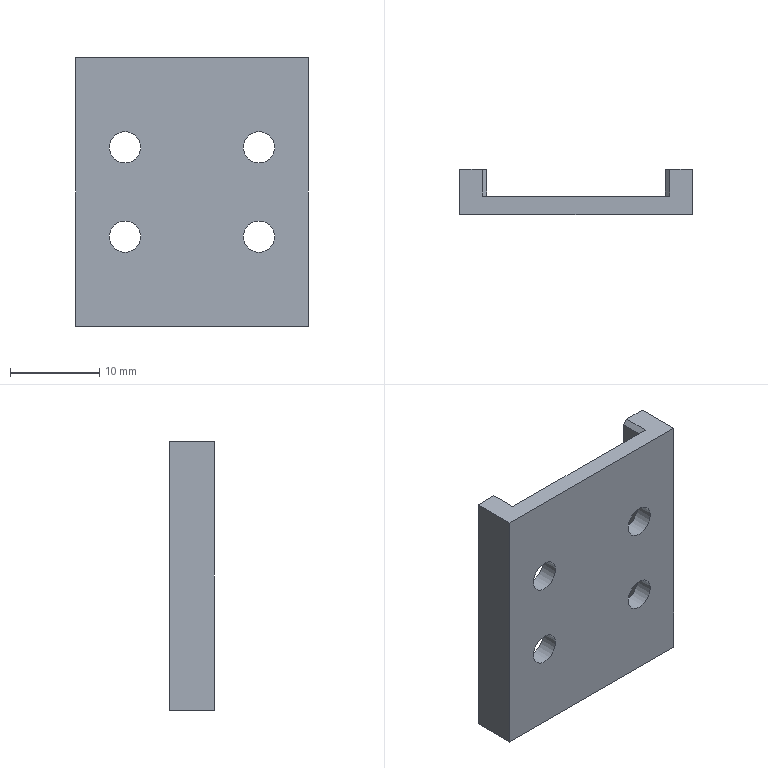Part | NX | 1 solid | 18 faces | box 26 x 5 x 30 mm | volume 2030 mm3 | plane 14 | cylinder 4 | commonest cylinder face diameters 3.5 x4
STEP:
#1=CARTESIAN_POINT('',(-13.,2.5,-15.));
#2=VERTEX_POINT('',#1);
#3=CARTESIAN_POINT('',(-13.,-2.5,-15.));
#4=VERTEX_POINT('',#3);
#5=CARTESIAN_POINT('',(-13.,2.5,-15.));
#6=DIRECTION('',(0.,-1.,0.));
#7=VECTOR('',#6,1000.);
#8=LINE('',#5,#7);
#9=EDGE_CURVE('',#2,#4,#8,.T.);
#10=ORIENTED_EDGE('',*,*,#9,.T.);
#11=CARTESIAN_POINT('',(-13.,-2.5,15.));
#12=VERTEX_POINT('',#11);
#13=CARTESIAN_POINT('',(-13.,-2.5,15.));
#14=DIRECTION('',(0.,0.,-1.));
#15=VECTOR('',#14,1000.);
#16=LINE('',#13,#15);
#17=EDGE_CURVE('',#12,#4,#16,.T.);
#18=ORIENTED_EDGE('',*,*,#17,.F.);
#19=CARTESIAN_POINT('',(-13.,2.5,15.));
#20=VERTEX_POINT('',#19);
#21=CARTESIAN_POINT('',(-13.,2.5,15.));
#22=DIRECTION('',(0.,-1.,0.));
#23=VECTOR('',#22,1000.);
#24=LINE('',#21,#23);
#25=EDGE_CURVE('',#20,#12,#24,.T.);
#26=ORIENTED_EDGE('',*,*,#25,.F.);
#27=CARTESIAN_POINT('',(-13.,2.5,15.));
#28=DIRECTION('',(0.,0.,-1.));
#29=VECTOR('',#28,1000.);
#30=LINE('',#27,#29);
#31=EDGE_CURVE('',#20,#2,#30,.T.);
#32=ORIENTED_EDGE('',*,*,#31,.T.);
#33=EDGE_LOOP('',(#10,#18,#26,#32));
#34=FACE_BOUND('',#33,.T.);
#35=CARTESIAN_POINT('',(-13.,2.5,15.));
#36=DIRECTION('',(1.,0.,0.));
#37=DIRECTION('',(0.,0.,-1.));
#38=AXIS2_PLACEMENT_3D('',#35,#36,#37);
#39=PLANE('',#38);
#40=ADVANCED_FACE('',(#34),#39,.F.);
#41=CARTESIAN_POINT('',(7.5,-2.5,-3.25));
#42=VERTEX_POINT('',#41);
#43=CARTESIAN_POINT('',(7.5,-2.5,-5.));
#44=DIRECTION('',(0.,1.,0.));
#45=DIRECTION('',(0.,0.,1.));
#46=AXIS2_PLACEMENT_3D('',#43,#44,#45);
#47=CIRCLE('',#46,1.75);
#48=EDGE_CURVE('',#42,#42,#47,.F.);
#49=ORIENTED_EDGE('',*,*,#48,.F.);
#50=EDGE_LOOP('',(#49));
#51=FACE_BOUND('',#50,.T.);
#52=CARTESIAN_POINT('',(-7.5,-2.5,6.75));
#53=VERTEX_POINT('',#52);
#54=CARTESIAN_POINT('',(-7.5,-2.5,5.));
#55=DIRECTION('',(0.,1.,0.));
#56=DIRECTION('',(0.,0.,1.));
#57=AXIS2_PLACEMENT_3D('',#54,#55,#56);
#58=CIRCLE('',#57,1.75);
#59=EDGE_CURVE('',#53,#53,#58,.F.);
#60=ORIENTED_EDGE('',*,*,#59,.F.);
#61=EDGE_LOOP('',(#60));
#62=FACE_BOUND('',#61,.T.);
#63=CARTESIAN_POINT('',(-7.5,-2.5,-3.25));
#64=VERTEX_POINT('',#63);
#65=CARTESIAN_POINT('',(-7.5,-2.5,-5.));
#66=DIRECTION('',(0.,1.,0.));
#67=DIRECTION('',(0.,0.,1.));
#68=AXIS2_PLACEMENT_3D('',#65,#66,#67);
#69=CIRCLE('',#68,1.75);
#70=EDGE_CURVE('',#64,#64,#69,.F.);
#71=ORIENTED_EDGE('',*,*,#70,.F.);
#72=EDGE_LOOP('',(#71));
#73=FACE_BOUND('',#72,.T.);
#74=CARTESIAN_POINT('',(7.5,-2.5,6.75));
#75=VERTEX_POINT('',#74);
#76=CARTESIAN_POINT('',(7.5,-2.5,5.));
#77=DIRECTION('',(0.,1.,0.));
#78=DIRECTION('',(0.,0.,1.));
#79=AXIS2_PLACEMENT_3D('',#76,#77,#78);
#80=CIRCLE('',#79,1.75);
#81=EDGE_CURVE('',#75,#75,#80,.F.);
#82=ORIENTED_EDGE('',*,*,#81,.F.);
#83=EDGE_LOOP('',(#82));
#84=FACE_BOUND('',#83,.T.);
#85=CARTESIAN_POINT('',(13.,-2.5,-15.));
#86=VERTEX_POINT('',#85);
#87=CARTESIAN_POINT('',(-13.,-2.5,-15.));
#88=DIRECTION('',(1.,0.,0.));
#89=VECTOR('',#88,1000.);
#90=LINE('',#87,#89);
#91=EDGE_CURVE('',#4,#86,#90,.T.);
#92=ORIENTED_EDGE('',*,*,#91,.T.);
#93=CARTESIAN_POINT('',(13.,-2.5,15.));
#94=VERTEX_POINT('',#93);
#95=CARTESIAN_POINT('',(13.,-2.5,15.));
#96=DIRECTION('',(0.,0.,-1.));
#97=VECTOR('',#96,1000.);
#98=LINE('',#95,#97);
#99=EDGE_CURVE('',#94,#86,#98,.T.);
#100=ORIENTED_EDGE('',*,*,#99,.F.);
#101=CARTESIAN_POINT('',(-13.,-2.5,15.));
#102=DIRECTION('',(1.,0.,0.));
#103=VECTOR('',#102,1000.);
#104=LINE('',#101,#103);
#105=EDGE_CURVE('',#12,#94,#104,.T.);
#106=ORIENTED_EDGE('',*,*,#105,.F.);
#107=ORIENTED_EDGE('',*,*,#17,.T.);
#108=EDGE_LOOP('',(#92,#100,#106,#107));
#109=FACE_BOUND('',#108,.T.);
#110=CARTESIAN_POINT('',(-13.,-2.5,15.));
#111=DIRECTION('',(0.,1.,0.));
#112=DIRECTION('',(0.,0.,1.));
#113=AXIS2_PLACEMENT_3D('',#110,#111,#112);
#114=PLANE('',#113);
#115=ADVANCED_FACE('',(#51,#62,#73,#84,#109),#114,.F.);
#116=CARTESIAN_POINT('',(13.,2.5,-15.));
#117=VERTEX_POINT('',#116);
#118=CARTESIAN_POINT('',(13.,-2.5,-15.));
#119=DIRECTION('',(0.,1.,0.));
#120=VECTOR('',#119,1000.);
#121=LINE('',#118,#120);
#122=EDGE_CURVE('',#86,#117,#121,.T.);
#123=ORIENTED_EDGE('',*,*,#122,.T.);
#124=CARTESIAN_POINT('',(13.,2.5,15.));
#125=VERTEX_POINT('',#124);
#126=CARTESIAN_POINT('',(13.,2.5,15.));
#127=DIRECTION('',(0.,0.,-1.));
#128=VECTOR('',#127,1000.);
#129=LINE('',#126,#128);
#130=EDGE_CURVE('',#125,#117,#129,.T.);
#131=ORIENTED_EDGE('',*,*,#130,.F.);
#132=CARTESIAN_POINT('',(13.,-2.5,15.));
#133=DIRECTION('',(0.,1.,0.));
#134=VECTOR('',#133,1000.);
#135=LINE('',#132,#134);
#136=EDGE_CURVE('',#94,#125,#135,.T.);
#137=ORIENTED_EDGE('',*,*,#136,.F.);
#138=ORIENTED_EDGE('',*,*,#99,.T.);
#139=EDGE_LOOP('',(#123,#131,#137,#138));
#140=FACE_BOUND('',#139,.T.);
#141=CARTESIAN_POINT('',(13.,-2.5,15.));
#142=DIRECTION('',(-1.,0.,0.));
#143=DIRECTION('',(0.,0.,1.));
#144=AXIS2_PLACEMENT_3D('',#141,#142,#143);
#145=PLANE('',#144);
#146=ADVANCED_FACE('',(#140),#145,.F.);
#147=CARTESIAN_POINT('',(10.5,2.5,-15.));
#148=VERTEX_POINT('',#147);
#149=CARTESIAN_POINT('',(13.,2.5,-15.));
#150=DIRECTION('',(-1.,0.,0.));
#151=VECTOR('',#150,1000.);
#152=LINE('',#149,#151);
#153=EDGE_CURVE('',#117,#148,#152,.T.);
#154=ORIENTED_EDGE('',*,*,#153,.T.);
#155=CARTESIAN_POINT('',(10.,2.5,-14.5));
#156=VERTEX_POINT('',#155);
#157=CARTESIAN_POINT('',(10.,2.5,-14.5));
#158=DIRECTION('',(0.7071,0.,-0.7071));
#159=VECTOR('',#158,1000.);
#160=LINE('',#157,#159);
#161=EDGE_CURVE('',#148,#156,#160,.F.);
#162=ORIENTED_EDGE('',*,*,#161,.T.);
#163=CARTESIAN_POINT('',(10.,2.5,14.5));
#164=VERTEX_POINT('',#163);
#165=CARTESIAN_POINT('',(10.,2.5,15.));
#166=DIRECTION('',(0.,0.,-1.));
#167=VECTOR('',#166,1000.);
#168=LINE('',#165,#167);
#169=EDGE_CURVE('',#164,#156,#168,.T.);
#170=ORIENTED_EDGE('',*,*,#169,.F.);
#171=CARTESIAN_POINT('',(10.5,2.5,15.));
#172=VERTEX_POINT('',#171);
#173=CARTESIAN_POINT('',(10.5,2.5,15.));
#174=DIRECTION('',(0.7071,0.,0.7071));
#175=VECTOR('',#174,1000.);
#176=LINE('',#173,#175);
#177=EDGE_CURVE('',#164,#172,#176,.T.);
#178=ORIENTED_EDGE('',*,*,#177,.T.);
#179=CARTESIAN_POINT('',(13.,2.5,15.));
#180=DIRECTION('',(-1.,0.,0.));
#181=VECTOR('',#180,1000.);
#182=LINE('',#179,#181);
#183=EDGE_CURVE('',#125,#172,#182,.T.);
#184=ORIENTED_EDGE('',*,*,#183,.F.);
#185=ORIENTED_EDGE('',*,*,#130,.T.);
#186=EDGE_LOOP('',(#154,#162,#170,#178,#184,#185));
#187=FACE_BOUND('',#186,.T.);
#188=CARTESIAN_POINT('',(13.,2.5,15.));
#189=DIRECTION('',(0.,-1.,0.));
#190=DIRECTION('',(0.,0.,-1.));
#191=AXIS2_PLACEMENT_3D('',#188,#189,#190);
#192=PLANE('',#191);
#193=ADVANCED_FACE('',(#187),#192,.F.);
#194=ORIENTED_EDGE('',*,*,#169,.T.);
#195=CARTESIAN_POINT('',(10.,-0.485,-14.5));
#196=VERTEX_POINT('',#195);
#197=CARTESIAN_POINT('',(10.,2.5,-14.5));
#198=DIRECTION('',(0.,-1.,0.));
#199=VECTOR('',#198,1000.);
#200=LINE('',#197,#199);
#201=EDGE_CURVE('',#156,#196,#200,.T.);
#202=ORIENTED_EDGE('',*,*,#201,.T.);
#203=CARTESIAN_POINT('',(10.,-0.485,14.5));
#204=VERTEX_POINT('',#203);
#205=CARTESIAN_POINT('',(10.,-0.485,15.));
#206=DIRECTION('',(0.,0.,-1.));
#207=VECTOR('',#206,1000.);
#208=LINE('',#205,#207);
#209=EDGE_CURVE('',#204,#196,#208,.T.);
#210=ORIENTED_EDGE('',*,*,#209,.F.);
#211=CARTESIAN_POINT('',(10.,2.5,14.5));
#212=DIRECTION('',(0.,1.,0.));
#213=VECTOR('',#212,1000.);
#214=LINE('',#211,#213);
#215=EDGE_CURVE('',#204,#164,#214,.T.);
#216=ORIENTED_EDGE('',*,*,#215,.T.);
#217=EDGE_LOOP('',(#194,#202,#210,#216));
#218=FACE_BOUND('',#217,.T.);
#219=CARTESIAN_POINT('',(10.,2.5,15.));
#220=DIRECTION('',(1.,0.,0.));
#221=DIRECTION('',(0.,1.,0.));
#222=AXIS2_PLACEMENT_3D('',#219,#220,#221);
#223=PLANE('',#222);
#224=ADVANCED_FACE('',(#218),#223,.F.);
#225=CARTESIAN_POINT('',(7.5,-0.485,-6.75));
#226=VERTEX_POINT('',#225);
#227=CARTESIAN_POINT('',(7.5,-0.485,-5.));
#228=DIRECTION('',(0.,-1.,0.));
#229=DIRECTION('',(0.,0.,-1.));
#230=AXIS2_PLACEMENT_3D('',#227,#228,#229);
#231=CIRCLE('',#230,1.75);
#232=EDGE_CURVE('',#226,#226,#231,.F.);
#233=ORIENTED_EDGE('',*,*,#232,.F.);
#234=EDGE_LOOP('',(#233));
#235=FACE_BOUND('',#234,.T.);
#236=CARTESIAN_POINT('',(-7.5,-0.485,3.25));
#237=VERTEX_POINT('',#236);
#238=CARTESIAN_POINT('',(-7.5,-0.485,5.));
#239=DIRECTION('',(0.,-1.,0.));
#240=DIRECTION('',(0.,0.,-1.));
#241=AXIS2_PLACEMENT_3D('',#238,#239,#240);
#242=CIRCLE('',#241,1.75);
#243=EDGE_CURVE('',#237,#237,#242,.F.);
#244=ORIENTED_EDGE('',*,*,#243,.F.);
#245=EDGE_LOOP('',(#244));
#246=FACE_BOUND('',#245,.T.);
#247=CARTESIAN_POINT('',(-7.5,-0.485,-6.75));
#248=VERTEX_POINT('',#247);
#249=CARTESIAN_POINT('',(-7.5,-0.485,-5.));
#250=DIRECTION('',(0.,-1.,0.));
#251=DIRECTION('',(0.,0.,-1.));
#252=AXIS2_PLACEMENT_3D('',#249,#250,#251);
#253=CIRCLE('',#252,1.75);
#254=EDGE_CURVE('',#248,#248,#253,.F.);
#255=ORIENTED_EDGE('',*,*,#254,.F.);
#256=EDGE_LOOP('',(#255));
#257=FACE_BOUND('',#256,.T.);
#258=CARTESIAN_POINT('',(7.5,-0.485,3.25));
#259=VERTEX_POINT('',#258);
#260=CARTESIAN_POINT('',(7.5,-0.485,5.));
#261=DIRECTION('',(0.,-1.,0.));
#262=DIRECTION('',(0.,0.,-1.));
#263=AXIS2_PLACEMENT_3D('',#260,#261,#262);
#264=CIRCLE('',#263,1.75);
#265=EDGE_CURVE('',#259,#259,#264,.F.);
#266=ORIENTED_EDGE('',*,*,#265,.F.);
#267=EDGE_LOOP('',(#266));
#268=FACE_BOUND('',#267,.T.);
#269=CARTESIAN_POINT('',(10.5,-0.485,-15.));
#270=VERTEX_POINT('',#269);
#271=CARTESIAN_POINT('',(-10.5,-0.485,-15.));
#272=VERTEX_POINT('',#271);
#273=CARTESIAN_POINT('',(10.,-0.485,-15.));
#274=DIRECTION('',(-1.,0.,0.));
#275=VECTOR('',#274,1000.);
#276=LINE('',#273,#275);
#277=EDGE_CURVE('',#270,#272,#276,.T.);
#278=ORIENTED_EDGE('',*,*,#277,.T.);
#279=CARTESIAN_POINT('',(-10.,-0.485,-14.5));
#280=VERTEX_POINT('',#279);
#281=CARTESIAN_POINT('',(14.75,-0.485,10.25));
#282=DIRECTION('',(-0.7071,0.,-0.7071));
#283=VECTOR('',#282,1000.);
#284=LINE('',#281,#283);
#285=EDGE_CURVE('',#272,#280,#284,.F.);
#286=ORIENTED_EDGE('',*,*,#285,.T.);
#287=CARTESIAN_POINT('',(-10.,-0.485,14.5));
#288=VERTEX_POINT('',#287);
#289=CARTESIAN_POINT('',(-10.,-0.485,15.));
#290=DIRECTION('',(0.,0.,-1.));
#291=VECTOR('',#290,1000.);
#292=LINE('',#289,#291);
#293=EDGE_CURVE('',#288,#280,#292,.T.);
#294=ORIENTED_EDGE('',*,*,#293,.F.);
#295=CARTESIAN_POINT('',(-10.5,-0.485,15.));
#296=VERTEX_POINT('',#295);
#297=CARTESIAN_POINT('',(-0.25,-0.485,4.75));
#298=DIRECTION('',(-0.7071,0.,0.7071));
#299=VECTOR('',#298,1000.);
#300=LINE('',#297,#299);
#301=EDGE_CURVE('',#288,#296,#300,.T.);
#302=ORIENTED_EDGE('',*,*,#301,.T.);
#303=CARTESIAN_POINT('',(10.5,-0.485,15.));
#304=VERTEX_POINT('',#303);
#305=CARTESIAN_POINT('',(10.,-0.485,15.));
#306=DIRECTION('',(-1.,0.,0.));
#307=VECTOR('',#306,1000.);
#308=LINE('',#305,#307);
#309=EDGE_CURVE('',#304,#296,#308,.T.);
#310=ORIENTED_EDGE('',*,*,#309,.F.);
#311=CARTESIAN_POINT('',(10.25,-0.485,14.75));
#312=DIRECTION('',(-0.7071,0.,-0.7071));
#313=VECTOR('',#312,1000.);
#314=LINE('',#311,#313);
#315=EDGE_CURVE('',#304,#204,#314,.T.);
#316=ORIENTED_EDGE('',*,*,#315,.T.);
#317=ORIENTED_EDGE('',*,*,#209,.T.);
#318=CARTESIAN_POINT('',(-4.75,-0.485,0.25));
#319=DIRECTION('',(-0.7071,0.,0.7071));
#320=VECTOR('',#319,1000.);
#321=LINE('',#318,#320);
#322=EDGE_CURVE('',#196,#270,#321,.F.);
#323=ORIENTED_EDGE('',*,*,#322,.T.);
#324=EDGE_LOOP('',(#278,#286,#294,#302,#310,#316,#317,#323));
#325=FACE_BOUND('',#324,.T.);
#326=CARTESIAN_POINT('',(10.,-0.485,15.));
#327=DIRECTION('',(0.,-1.,0.));
#328=DIRECTION('',(0.,0.,-1.));
#329=AXIS2_PLACEMENT_3D('',#326,#327,#328);
#330=PLANE('',#329);
#331=ADVANCED_FACE('',(#235,#246,#257,#268,#325),#330,.F.);
#332=ORIENTED_EDGE('',*,*,#293,.T.);
#333=CARTESIAN_POINT('',(-10.,2.5,-14.5));
#334=VERTEX_POINT('',#333);
#335=CARTESIAN_POINT('',(-10.,-0.485,-14.5));
#336=DIRECTION('',(0.,1.,0.));
#337=VECTOR('',#336,1000.);
#338=LINE('',#335,#337);
#339=EDGE_CURVE('',#280,#334,#338,.T.);
#340=ORIENTED_EDGE('',*,*,#339,.T.);
#341=CARTESIAN_POINT('',(-10.,2.5,14.5));
#342=VERTEX_POINT('',#341);
#343=CARTESIAN_POINT('',(-10.,2.5,15.));
#344=DIRECTION('',(0.,0.,-1.));
#345=VECTOR('',#344,1000.);
#346=LINE('',#343,#345);
#347=EDGE_CURVE('',#342,#334,#346,.T.);
#348=ORIENTED_EDGE('',*,*,#347,.F.);
#349=CARTESIAN_POINT('',(-10.,-0.485,14.5));
#350=DIRECTION('',(0.,-1.,0.));
#351=VECTOR('',#350,1000.);
#352=LINE('',#349,#351);
#353=EDGE_CURVE('',#342,#288,#352,.T.);
#354=ORIENTED_EDGE('',*,*,#353,.T.);
#355=EDGE_LOOP('',(#332,#340,#348,#354));
#356=FACE_BOUND('',#355,.T.);
#357=CARTESIAN_POINT('',(-10.,-0.485,15.));
#358=DIRECTION('',(-1.,0.,0.));
#359=DIRECTION('',(0.,-1.,0.));
#360=AXIS2_PLACEMENT_3D('',#357,#358,#359);
#361=PLANE('',#360);
#362=ADVANCED_FACE('',(#356),#361,.F.);
#363=ORIENTED_EDGE('',*,*,#347,.T.);
#364=CARTESIAN_POINT('',(-10.5,2.5,-15.));
#365=VERTEX_POINT('',#364);
#366=CARTESIAN_POINT('',(-10.,2.5,-14.5));
#367=DIRECTION('',(0.7071,0.,0.7071));
#368=VECTOR('',#367,1000.);
#369=LINE('',#366,#368);
#370=EDGE_CURVE('',#334,#365,#369,.F.);
#371=ORIENTED_EDGE('',*,*,#370,.T.);
#372=CARTESIAN_POINT('',(-10.,2.5,-15.));
#373=DIRECTION('',(-1.,0.,0.));
#374=VECTOR('',#373,1000.);
#375=LINE('',#372,#374);
#376=EDGE_CURVE('',#365,#2,#375,.T.);
#377=ORIENTED_EDGE('',*,*,#376,.T.);
#378=ORIENTED_EDGE('',*,*,#31,.F.);
#379=CARTESIAN_POINT('',(-10.5,2.5,15.));
#380=VERTEX_POINT('',#379);
#381=CARTESIAN_POINT('',(-10.,2.5,15.));
#382=DIRECTION('',(-1.,0.,0.));
#383=VECTOR('',#382,1000.);
#384=LINE('',#381,#383);
#385=EDGE_CURVE('',#380,#20,#384,.T.);
#386=ORIENTED_EDGE('',*,*,#385,.F.);
#387=CARTESIAN_POINT('',(-10.5,2.5,15.));
#388=DIRECTION('',(0.7071,0.,-0.7071));
#389=VECTOR('',#388,1000.);
#390=LINE('',#387,#389);
#391=EDGE_CURVE('',#380,#342,#390,.T.);
#392=ORIENTED_EDGE('',*,*,#391,.T.);
#393=EDGE_LOOP('',(#363,#371,#377,#378,#386,#392));
#394=FACE_BOUND('',#393,.T.);
#395=CARTESIAN_POINT('',(-10.,2.5,15.));
#396=DIRECTION('',(0.,-1.,0.));
#397=DIRECTION('',(0.,0.,-1.));
#398=AXIS2_PLACEMENT_3D('',#395,#396,#397);
#399=PLANE('',#398);
#400=ADVANCED_FACE('',(#394),#399,.F.);
#401=ORIENTED_EDGE('',*,*,#183,.T.);
#402=CARTESIAN_POINT('',(10.5,-0.485,15.));
#403=DIRECTION('',(0.,-1.,0.));
#404=VECTOR('',#403,1000.);
#405=LINE('',#402,#404);
#406=EDGE_CURVE('',#172,#304,#405,.T.);
#407=ORIENTED_EDGE('',*,*,#406,.T.);
#408=ORIENTED_EDGE('',*,*,#309,.T.);
#409=CARTESIAN_POINT('',(-10.5,2.5,15.));
#410=DIRECTION('',(0.,1.,0.));
#411=VECTOR('',#410,1000.);
#412=LINE('',#409,#411);
#413=EDGE_CURVE('',#296,#380,#412,.T.);
#414=ORIENTED_EDGE('',*,*,#413,.T.);
#415=ORIENTED_EDGE('',*,*,#385,.T.);
#416=ORIENTED_EDGE('',*,*,#25,.T.);
#417=ORIENTED_EDGE('',*,*,#105,.T.);
#418=ORIENTED_EDGE('',*,*,#136,.T.);
#419=EDGE_LOOP('',(#401,#407,#408,#414,#415,#416,#417,#418));
#420=FACE_BOUND('',#419,.T.);
#421=CARTESIAN_POINT('',(0.,0.,15.));
#422=DIRECTION('',(0.,0.,1.));
#423=DIRECTION('',(1.,0.,0.));
#424=AXIS2_PLACEMENT_3D('',#421,#422,#423);
#425=PLANE('',#424);
#426=ADVANCED_FACE('',(#420),#425,.T.);
#427=ORIENTED_EDGE('',*,*,#277,.F.);
#428=CARTESIAN_POINT('',(10.5,0.,-15.));
#429=DIRECTION('',(0.,1.,0.));
#430=VECTOR('',#429,1000.);
#431=LINE('',#428,#430);
#432=EDGE_CURVE('',#270,#148,#431,.T.);
#433=ORIENTED_EDGE('',*,*,#432,.T.);
#434=ORIENTED_EDGE('',*,*,#153,.F.);
#435=ORIENTED_EDGE('',*,*,#122,.F.);
#436=ORIENTED_EDGE('',*,*,#91,.F.);
#437=ORIENTED_EDGE('',*,*,#9,.F.);
#438=ORIENTED_EDGE('',*,*,#376,.F.);
#439=CARTESIAN_POINT('',(-10.5,0.,-15.));
#440=DIRECTION('',(0.,-1.,0.));
#441=VECTOR('',#440,1000.);
#442=LINE('',#439,#441);
#443=EDGE_CURVE('',#365,#272,#442,.T.);
#444=ORIENTED_EDGE('',*,*,#443,.T.);
#445=EDGE_LOOP('',(#427,#433,#434,#435,#436,#437,#438,#444));
#446=FACE_BOUND('',#445,.T.);
#447=CARTESIAN_POINT('',(0.,0.,-15.));
#448=DIRECTION('',(0.,0.,1.));
#449=DIRECTION('',(1.,0.,0.));
#450=AXIS2_PLACEMENT_3D('',#447,#448,#449);
#451=PLANE('',#450);
#452=ADVANCED_FACE('',(#446),#451,.F.);
#453=ORIENTED_EDGE('',*,*,#265,.T.);
#454=EDGE_LOOP('',(#453));
#455=FACE_BOUND('',#454,.T.);
#456=ORIENTED_EDGE('',*,*,#81,.T.);
#457=EDGE_LOOP('',(#456));
#458=FACE_BOUND('',#457,.T.);
#459=CARTESIAN_POINT('',(7.5,14.515,5.));
#460=DIRECTION('',(0.,-1.,0.));
#461=DIRECTION('',(0.,0.,-1.));
#462=AXIS2_PLACEMENT_3D('',#459,#460,#461);
#463=CYLINDRICAL_SURFACE('',#462,1.75);
#464=ADVANCED_FACE('',(#455,#458),#463,.F.);
#465=ORIENTED_EDGE('',*,*,#254,.T.);
#466=EDGE_LOOP('',(#465));
#467=FACE_BOUND('',#466,.T.);
#468=ORIENTED_EDGE('',*,*,#70,.T.);
#469=EDGE_LOOP('',(#468));
#470=FACE_BOUND('',#469,.T.);
#471=CARTESIAN_POINT('',(-7.5,14.515,-5.));
#472=DIRECTION('',(0.,-1.,0.));
#473=DIRECTION('',(0.,0.,-1.));
#474=AXIS2_PLACEMENT_3D('',#471,#472,#473);
#475=CYLINDRICAL_SURFACE('',#474,1.75);
#476=ADVANCED_FACE('',(#467,#470),#475,.F.);
#477=ORIENTED_EDGE('',*,*,#243,.T.);
#478=EDGE_LOOP('',(#477));
#479=FACE_BOUND('',#478,.T.);
#480=ORIENTED_EDGE('',*,*,#59,.T.);
#481=EDGE_LOOP('',(#480));
#482=FACE_BOUND('',#481,.T.);
#483=CARTESIAN_POINT('',(-7.5,14.515,5.));
#484=DIRECTION('',(0.,-1.,0.));
#485=DIRECTION('',(0.,0.,-1.));
#486=AXIS2_PLACEMENT_3D('',#483,#484,#485);
#487=CYLINDRICAL_SURFACE('',#486,1.75);
#488=ADVANCED_FACE('',(#479,#482),#487,.F.);
#489=ORIENTED_EDGE('',*,*,#232,.T.);
#490=EDGE_LOOP('',(#489));
#491=FACE_BOUND('',#490,.T.);
#492=ORIENTED_EDGE('',*,*,#48,.T.);
#493=EDGE_LOOP('',(#492));
#494=FACE_BOUND('',#493,.T.);
#495=CARTESIAN_POINT('',(7.5,14.515,-5.));
#496=DIRECTION('',(0.,-1.,0.));
#497=DIRECTION('',(0.,0.,-1.));
#498=AXIS2_PLACEMENT_3D('',#495,#496,#497);
#499=CYLINDRICAL_SURFACE('',#498,1.75);
#500=ADVANCED_FACE('',(#491,#494),#499,.F.);
#501=ORIENTED_EDGE('',*,*,#161,.F.);
#502=ORIENTED_EDGE('',*,*,#432,.F.);
#503=ORIENTED_EDGE('',*,*,#322,.F.);
#504=ORIENTED_EDGE('',*,*,#201,.F.);
#505=EDGE_LOOP('',(#501,#502,#503,#504));
#506=FACE_BOUND('',#505,.T.);
#507=CARTESIAN_POINT('',(10.,2.5,-14.5));
#508=DIRECTION('',(0.7071,0.,0.7071));
#509=DIRECTION('',(0.,-1.,0.));
#510=AXIS2_PLACEMENT_3D('',#507,#508,#509);
#511=PLANE('',#510);
#512=ADVANCED_FACE('',(#506),#511,.F.);
#513=ORIENTED_EDGE('',*,*,#177,.F.);
#514=ORIENTED_EDGE('',*,*,#215,.F.);
#515=ORIENTED_EDGE('',*,*,#315,.F.);
#516=ORIENTED_EDGE('',*,*,#406,.F.);
#517=EDGE_LOOP('',(#513,#514,#515,#516));
#518=FACE_BOUND('',#517,.T.);
#519=CARTESIAN_POINT('',(10.5,0.,15.));
#520=DIRECTION('',(-0.7071,0.,0.7071));
#521=DIRECTION('',(0.,1.,0.));
#522=AXIS2_PLACEMENT_3D('',#519,#520,#521);
#523=PLANE('',#522);
#524=ADVANCED_FACE('',(#518),#523,.T.);
#525=ORIENTED_EDGE('',*,*,#285,.F.);
#526=ORIENTED_EDGE('',*,*,#443,.F.);
#527=ORIENTED_EDGE('',*,*,#370,.F.);
#528=ORIENTED_EDGE('',*,*,#339,.F.);
#529=EDGE_LOOP('',(#525,#526,#527,#528));
#530=FACE_BOUND('',#529,.T.);
#531=CARTESIAN_POINT('',(-10.,-0.485,-14.5));
#532=DIRECTION('',(-0.7071,0.,0.7071));
#533=DIRECTION('',(0.,1.,0.));
#534=AXIS2_PLACEMENT_3D('',#531,#532,#533);
#535=PLANE('',#534);
#536=ADVANCED_FACE('',(#530),#535,.F.);
#537=ORIENTED_EDGE('',*,*,#301,.F.);
#538=ORIENTED_EDGE('',*,*,#353,.F.);
#539=ORIENTED_EDGE('',*,*,#391,.F.);
#540=ORIENTED_EDGE('',*,*,#413,.F.);
#541=EDGE_LOOP('',(#537,#538,#539,#540));
#542=FACE_BOUND('',#541,.T.);
#543=CARTESIAN_POINT('',(-10.5,0.,15.));
#544=DIRECTION('',(0.7071,0.,0.7071));
#545=DIRECTION('',(0.,-1.,0.));
#546=AXIS2_PLACEMENT_3D('',#543,#544,#545);
#547=PLANE('',#546);
#548=ADVANCED_FACE('',(#542),#547,.T.);
#549=CLOSED_SHELL('',(#40,#115,#146,#193,#224,#331,#362,#400,#426,#452,#464,#476,#488,#500,#512,#524,#536,#548));
#550=MANIFOLD_SOLID_BREP('',#549);
#551=(LENGTH_UNIT()NAMED_UNIT(*)SI_UNIT(.MILLI.,.METRE.));
#552=UNCERTAINTY_MEASURE_WITH_UNIT(LENGTH_MEASURE(0.00001),#551,'','');
#553=(NAMED_UNIT(*)PLANE_ANGLE_UNIT()SI_UNIT($,.RADIAN.));
#554=(NAMED_UNIT(*)SI_UNIT($,.STERADIAN.)SOLID_ANGLE_UNIT());
#555=(GEOMETRIC_REPRESENTATION_CONTEXT(3)GLOBAL_UNCERTAINTY_ASSIGNED_CONTEXT((#552))GLOBAL_UNIT_ASSIGNED_CONTEXT((#551,#553,#554))REPRESENTATION_CONTEXT('',''));
#556=ADVANCED_BREP_SHAPE_REPRESENTATION('',(#550),#555);